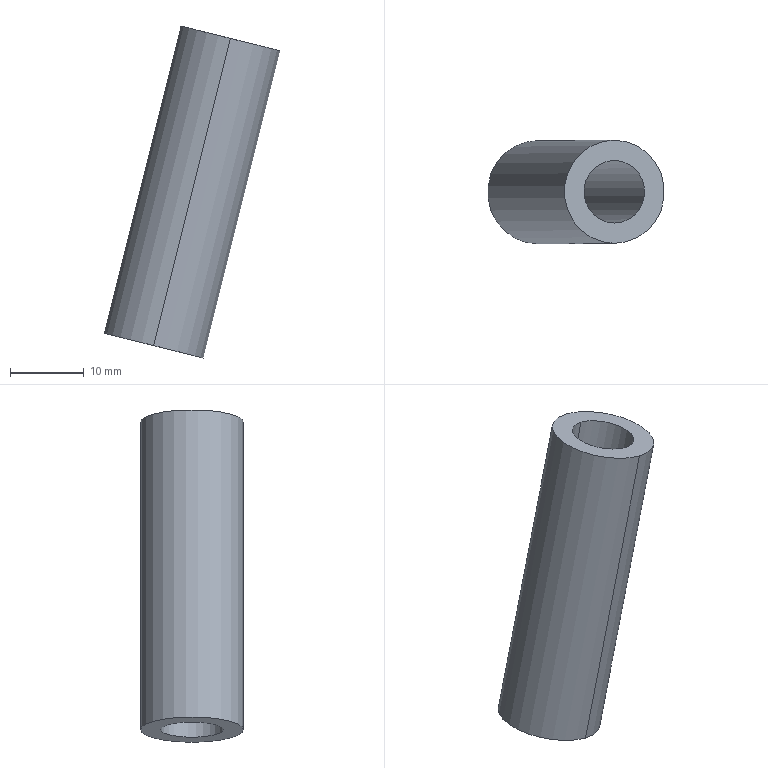Part | SolidWorks | features BaseBody 1 | 1 solid | 6 faces | box 23.985 x 14 x 45.109 mm | volume 4179 mm3 | cylinder 4 | plane 2 | commonest cylinder face diameters 8.5 x2 14 x2
STEP:
#1=CARTESIAN_POINT('',(-480.545,-52.608,231.824));
#2=VERTEX_POINT('',#1);
#3=CARTESIAN_POINT('',(-480.545,-61.108,231.824));
#4=VERTEX_POINT('',#3);
#5=CARTESIAN_POINT('',(-480.545,-56.858,231.824));
#6=DIRECTION('',(-0.2419,0.,-0.9703));
#7=DIRECTION('',(0.9703,0.,-0.2419));
#8=AXIS2_PLACEMENT_3D('',#5,#6,#7);
#9=CIRCLE('',#8,4.25);
#10=EDGE_CURVE('',#2,#4,#9,.T.);
#11=ORIENTED_EDGE('',*,*,#10,.T.);
#12=CARTESIAN_POINT('',(-470.144,-61.108,273.547));
#13=VERTEX_POINT('',#12);
#14=CARTESIAN_POINT('',(-475.708,-61.108,251.23));
#15=DIRECTION('',(0.2419,0.,0.9703));
#16=VECTOR('',#15,1000.);
#17=LINE('',#14,#16);
#18=EDGE_CURVE('',#4,#13,#17,.T.);
#19=ORIENTED_EDGE('',*,*,#18,.T.);
#20=CARTESIAN_POINT('',(-470.144,-52.608,273.547));
#21=VERTEX_POINT('',#20);
#22=CARTESIAN_POINT('',(-470.144,-56.858,273.547));
#23=DIRECTION('',(0.2419,0.,0.9703));
#24=DIRECTION('',(0.9703,0.,-0.2419));
#25=AXIS2_PLACEMENT_3D('',#22,#23,#24);
#26=CIRCLE('',#25,4.25);
#27=EDGE_CURVE('',#13,#21,#26,.T.);
#28=ORIENTED_EDGE('',*,*,#27,.T.);
#29=CARTESIAN_POINT('',(-475.708,-52.608,251.23));
#30=DIRECTION('',(0.2419,0.,0.9703));
#31=VECTOR('',#30,1000.);
#32=LINE('',#29,#31);
#33=EDGE_CURVE('',#2,#21,#32,.T.);
#34=ORIENTED_EDGE('',*,*,#33,.F.);
#35=EDGE_LOOP('',(#11,#19,#28,#34));
#36=FACE_OUTER_BOUND('',#35,.T.);
#37=CARTESIAN_POINT('',(-475.708,-56.858,251.23));
#38=DIRECTION('',(0.2419,0.,0.9703));
#39=DIRECTION('',(0.,1.,0.));
#40=AXIS2_PLACEMENT_3D('',#37,#38,#39);
#41=CYLINDRICAL_SURFACE('',#40,4.25);
#42=ADVANCED_FACE('',(#36),#41,.F.);
#43=CARTESIAN_POINT('',(-480.545,-49.858,231.824));
#44=VERTEX_POINT('',#43);
#45=CARTESIAN_POINT('',(-480.545,-63.858,231.824));
#46=VERTEX_POINT('',#45);
#47=CARTESIAN_POINT('',(-480.545,-56.858,231.824));
#48=DIRECTION('',(0.2419,0.,0.9703));
#49=DIRECTION('',(0.9703,0.,-0.2419));
#50=AXIS2_PLACEMENT_3D('',#47,#48,#49);
#51=CIRCLE('',#50,7.);
#52=EDGE_CURVE('',#44,#46,#51,.T.);
#53=ORIENTED_EDGE('',*,*,#52,.T.);
#54=CARTESIAN_POINT('',(-470.144,-63.858,273.547));
#55=VERTEX_POINT('',#54);
#56=CARTESIAN_POINT('',(-475.708,-63.858,251.23));
#57=DIRECTION('',(0.2419,0.,0.9703));
#58=VECTOR('',#57,1000.);
#59=LINE('',#56,#58);
#60=EDGE_CURVE('',#46,#55,#59,.T.);
#61=ORIENTED_EDGE('',*,*,#60,.T.);
#62=CARTESIAN_POINT('',(-470.144,-49.858,273.547));
#63=VERTEX_POINT('',#62);
#64=CARTESIAN_POINT('',(-470.144,-56.858,273.547));
#65=DIRECTION('',(0.2419,0.,0.9703));
#66=DIRECTION('',(0.9703,0.,-0.2419));
#67=AXIS2_PLACEMENT_3D('',#64,#65,#66);
#68=CIRCLE('',#67,7.);
#69=EDGE_CURVE('',#63,#55,#68,.T.);
#70=ORIENTED_EDGE('',*,*,#69,.F.);
#71=CARTESIAN_POINT('',(-475.708,-49.858,251.23));
#72=DIRECTION('',(0.2419,0.,0.9703));
#73=VECTOR('',#72,1000.);
#74=LINE('',#71,#73);
#75=EDGE_CURVE('',#44,#63,#74,.T.);
#76=ORIENTED_EDGE('',*,*,#75,.F.);
#77=EDGE_LOOP('',(#53,#61,#70,#76));
#78=FACE_OUTER_BOUND('',#77,.T.);
#79=CARTESIAN_POINT('',(-475.708,-56.858,251.23));
#80=DIRECTION('',(0.2419,0.,0.9703));
#81=DIRECTION('',(0.,1.,0.));
#82=AXIS2_PLACEMENT_3D('',#79,#80,#81);
#83=CYLINDRICAL_SURFACE('',#82,7.);
#84=ADVANCED_FACE('',(#78),#83,.T.);
#85=ORIENTED_EDGE('',*,*,#10,.F.);
#86=CARTESIAN_POINT('',(-480.545,-56.858,231.824));
#87=DIRECTION('',(-0.2419,0.,-0.9703));
#88=DIRECTION('',(0.9703,0.,-0.2419));
#89=AXIS2_PLACEMENT_3D('',#86,#87,#88);
#90=CIRCLE('',#89,4.25);
#91=EDGE_CURVE('',#4,#2,#90,.T.);
#92=ORIENTED_EDGE('',*,*,#91,.F.);
#93=EDGE_LOOP('',(#85,#92));
#94=FACE_BOUND('',#93,.T.);
#95=ORIENTED_EDGE('',*,*,#52,.F.);
#96=CARTESIAN_POINT('',(-480.545,-56.858,231.824));
#97=DIRECTION('',(0.2419,0.,0.9703));
#98=DIRECTION('',(0.9703,0.,-0.2419));
#99=AXIS2_PLACEMENT_3D('',#96,#97,#98);
#100=CIRCLE('',#99,7.);
#101=EDGE_CURVE('',#46,#44,#100,.T.);
#102=ORIENTED_EDGE('',*,*,#101,.F.);
#103=EDGE_LOOP('',(#95,#102));
#104=FACE_OUTER_BOUND('',#103,.T.);
#105=CARTESIAN_POINT('',(-428.628,-66.,218.882));
#106=DIRECTION('',(0.2419,0.,0.9703));
#107=DIRECTION('',(0.,-1.,0.));
#108=AXIS2_PLACEMENT_3D('',#105,#106,#107);
#109=PLANE('',#108);
#110=ADVANCED_FACE('',(#94,#104),#109,.F.);
#111=CARTESIAN_POINT('',(-470.144,-56.858,273.547));
#112=DIRECTION('',(0.2419,0.,0.9703));
#113=DIRECTION('',(0.9703,0.,-0.2419));
#114=AXIS2_PLACEMENT_3D('',#111,#112,#113);
#115=CIRCLE('',#114,4.25);
#116=EDGE_CURVE('',#21,#13,#115,.T.);
#117=ORIENTED_EDGE('',*,*,#116,.F.);
#118=ORIENTED_EDGE('',*,*,#27,.F.);
#119=EDGE_LOOP('',(#117,#118));
#120=FACE_BOUND('',#119,.T.);
#121=ORIENTED_EDGE('',*,*,#69,.T.);
#122=CARTESIAN_POINT('',(-470.144,-56.858,273.547));
#123=DIRECTION('',(0.2419,0.,0.9703));
#124=DIRECTION('',(0.9703,0.,-0.2419));
#125=AXIS2_PLACEMENT_3D('',#122,#123,#124);
#126=CIRCLE('',#125,7.);
#127=EDGE_CURVE('',#55,#63,#126,.T.);
#128=ORIENTED_EDGE('',*,*,#127,.T.);
#129=EDGE_LOOP('',(#121,#128));
#130=FACE_OUTER_BOUND('',#129,.T.);
#131=CARTESIAN_POINT('',(-418.227,-66.,260.605));
#132=DIRECTION('',(0.2419,0.,0.9703));
#133=DIRECTION('',(0.,-1.,0.));
#134=AXIS2_PLACEMENT_3D('',#131,#132,#133);
#135=PLANE('',#134);
#136=ADVANCED_FACE('',(#120,#130),#135,.T.);
#137=ORIENTED_EDGE('',*,*,#60,.F.);
#138=ORIENTED_EDGE('',*,*,#101,.T.);
#139=ORIENTED_EDGE('',*,*,#75,.T.);
#140=ORIENTED_EDGE('',*,*,#127,.F.);
#141=EDGE_LOOP('',(#137,#138,#139,#140));
#142=FACE_OUTER_BOUND('',#141,.T.);
#143=CARTESIAN_POINT('',(-475.708,-56.858,251.23));
#144=DIRECTION('',(0.2419,0.,0.9703));
#145=DIRECTION('',(0.,1.,0.));
#146=AXIS2_PLACEMENT_3D('',#143,#144,#145);
#147=CYLINDRICAL_SURFACE('',#146,7.);
#148=ADVANCED_FACE('',(#142),#147,.T.);
#149=ORIENTED_EDGE('',*,*,#18,.F.);
#150=ORIENTED_EDGE('',*,*,#91,.T.);
#151=ORIENTED_EDGE('',*,*,#33,.T.);
#152=ORIENTED_EDGE('',*,*,#116,.T.);
#153=EDGE_LOOP('',(#149,#150,#151,#152));
#154=FACE_OUTER_BOUND('',#153,.T.);
#155=CARTESIAN_POINT('',(-475.708,-56.858,251.23));
#156=DIRECTION('',(0.2419,0.,0.9703));
#157=DIRECTION('',(0.,1.,0.));
#158=AXIS2_PLACEMENT_3D('',#155,#156,#157);
#159=CYLINDRICAL_SURFACE('',#158,4.25);
#160=ADVANCED_FACE('',(#154),#159,.F.);
#161=CLOSED_SHELL('',(#42,#84,#110,#136,#148,#160));
#162=MANIFOLD_SOLID_BREP('',#161);
#163=CARTESIAN_POINT('',(0.,0.,0.));
#164=DIRECTION('',(0.,0.,1.));
#165=DIRECTION('',(1.,0.,0.));
#166=AXIS2_PLACEMENT_3D('',#163,#164,#165);
#167=(LENGTH_UNIT()NAMED_UNIT(*)SI_UNIT(.MILLI.,.METRE.));
#168=UNCERTAINTY_MEASURE_WITH_UNIT(LENGTH_MEASURE(0.00001),#167,'','');
#169=(NAMED_UNIT(*)PLANE_ANGLE_UNIT()SI_UNIT($,.RADIAN.));
#170=(NAMED_UNIT(*)SI_UNIT($,.STERADIAN.)SOLID_ANGLE_UNIT());
#171=(GEOMETRIC_REPRESENTATION_CONTEXT(3)GLOBAL_UNCERTAINTY_ASSIGNED_CONTEXT((#168))GLOBAL_UNIT_ASSIGNED_CONTEXT((#167,#169,#170))REPRESENTATION_CONTEXT('',''));
#172=ADVANCED_BREP_SHAPE_REPRESENTATION('',(#162,#166),#171);